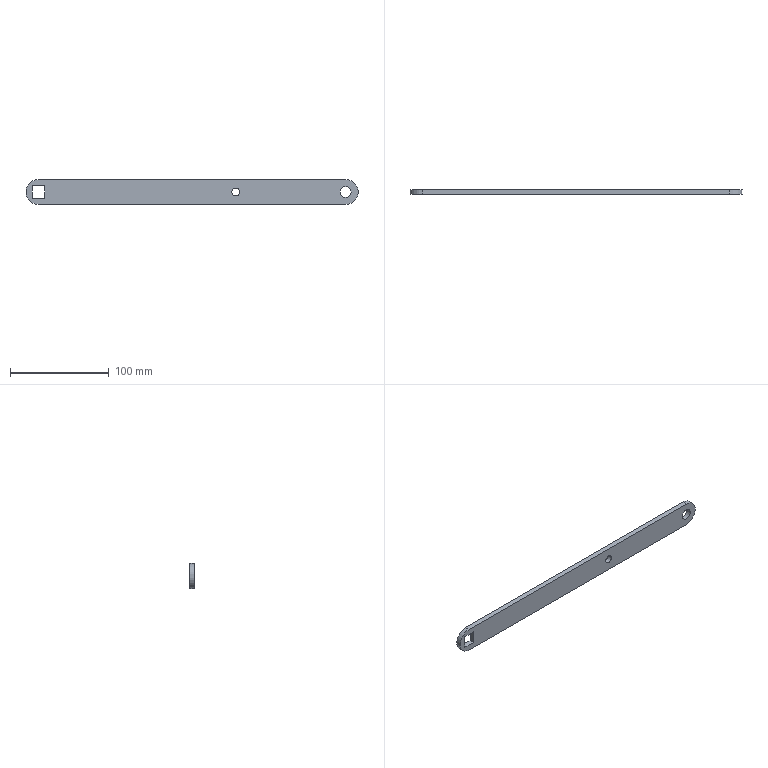Part | NX | features BREP 1 | 1 solid | 18 faces | box 336.55 x 4.763 x 25.4 mm | volume 38541 mm3 | cylinder 10 | plane 8 | commonest cylinder face diameters 0.762 x4 8.128 x2 11.151 x2 25.4 x2
STEP:
#1=CARTESIAN_POINT('',(-155.575,0.,12.7));
#2=VERTEX_POINT('',#1);
#3=CARTESIAN_POINT('',(155.575,0.,12.7));
#4=VERTEX_POINT('',#3);
#5=CARTESIAN_POINT('',(-155.575,0.,12.7));
#6=DIRECTION('',(1.,0.,0.));
#7=VECTOR('',#6,1000.);
#8=LINE('',#5,#7);
#9=EDGE_CURVE('',#2,#4,#8,.T.);
#10=ORIENTED_EDGE('',*,*,#9,.T.);
#11=CARTESIAN_POINT('',(155.575,0.,-12.7));
#12=VERTEX_POINT('',#11);
#13=CARTESIAN_POINT('',(155.575,0.,0.));
#14=DIRECTION('',(0.,1.,0.));
#15=DIRECTION('',(0.,0.,1.));
#16=AXIS2_PLACEMENT_3D('',#13,#14,#15);
#17=CIRCLE('',#16,12.7);
#18=EDGE_CURVE('',#4,#12,#17,.T.);
#19=ORIENTED_EDGE('',*,*,#18,.T.);
#20=CARTESIAN_POINT('',(-155.575,0.,-12.7));
#21=VERTEX_POINT('',#20);
#22=CARTESIAN_POINT('',(155.575,0.,-12.7));
#23=DIRECTION('',(-1.,0.,0.));
#24=VECTOR('',#23,1000.);
#25=LINE('',#22,#24);
#26=EDGE_CURVE('',#12,#21,#25,.T.);
#27=ORIENTED_EDGE('',*,*,#26,.T.);
#28=CARTESIAN_POINT('',(-155.575,0.,0.));
#29=DIRECTION('',(0.,1.,0.));
#30=DIRECTION('',(0.,0.,-1.));
#31=AXIS2_PLACEMENT_3D('',#28,#29,#30);
#32=CIRCLE('',#31,12.7);
#33=EDGE_CURVE('',#21,#2,#32,.T.);
#34=ORIENTED_EDGE('',*,*,#33,.T.);
#35=EDGE_LOOP('',(#10,#19,#27,#34));
#36=FACE_BOUND('',#35,.T.);
#37=CARTESIAN_POINT('',(150.,0.,0.));
#38=VERTEX_POINT('',#37);
#39=CARTESIAN_POINT('',(161.15,0.,0.));
#40=VERTEX_POINT('',#39);
#41=CARTESIAN_POINT('',(155.575,0.,0.));
#42=DIRECTION('',(0.,-1.,0.));
#43=DIRECTION('',(-1.,0.,0.));
#44=AXIS2_PLACEMENT_3D('',#41,#42,#43);
#45=CIRCLE('',#44,5.575);
#46=EDGE_CURVE('',#38,#40,#45,.T.);
#47=ORIENTED_EDGE('',*,*,#46,.T.);
#48=CARTESIAN_POINT('',(155.575,0.,0.));
#49=DIRECTION('',(0.,-1.,0.));
#50=DIRECTION('',(1.,0.,0.));
#51=AXIS2_PLACEMENT_3D('',#48,#49,#50);
#52=CIRCLE('',#51,5.575);
#53=EDGE_CURVE('',#40,#38,#52,.T.);
#54=ORIENTED_EDGE('',*,*,#53,.T.);
#55=EDGE_LOOP('',(#47,#54));
#56=FACE_BOUND('',#55,.T.);
#57=CARTESIAN_POINT('',(-149.098,0.,6.096));
#58=VERTEX_POINT('',#57);
#59=CARTESIAN_POINT('',(-149.479,0.,6.477));
#60=VERTEX_POINT('',#59);
#61=CARTESIAN_POINT('',(-149.479,0.,6.096));
#62=DIRECTION('',(0.,-1.,0.));
#63=DIRECTION('',(1.,0.,0.));
#64=AXIS2_PLACEMENT_3D('',#61,#62,#63);
#65=CIRCLE('',#64,0.381);
#66=EDGE_CURVE('',#58,#60,#65,.T.);
#67=ORIENTED_EDGE('',*,*,#66,.T.);
#68=CARTESIAN_POINT('',(-161.671,0.,6.477));
#69=VERTEX_POINT('',#68);
#70=CARTESIAN_POINT('',(-149.479,0.,6.477));
#71=DIRECTION('',(-1.,0.,0.));
#72=VECTOR('',#71,1000.);
#73=LINE('',#70,#72);
#74=EDGE_CURVE('',#60,#69,#73,.T.);
#75=ORIENTED_EDGE('',*,*,#74,.T.);
#76=CARTESIAN_POINT('',(-162.052,0.,6.096));
#77=VERTEX_POINT('',#76);
#78=CARTESIAN_POINT('',(-161.671,0.,6.096));
#79=DIRECTION('',(0.,-1.,0.));
#80=DIRECTION('',(0.,0.,1.));
#81=AXIS2_PLACEMENT_3D('',#78,#79,#80);
#82=CIRCLE('',#81,0.381);
#83=EDGE_CURVE('',#69,#77,#82,.T.);
#84=ORIENTED_EDGE('',*,*,#83,.T.);
#85=CARTESIAN_POINT('',(-162.052,0.,-6.096));
#86=VERTEX_POINT('',#85);
#87=CARTESIAN_POINT('',(-162.052,0.,6.096));
#88=DIRECTION('',(0.,0.,-1.));
#89=VECTOR('',#88,1000.);
#90=LINE('',#87,#89);
#91=EDGE_CURVE('',#77,#86,#90,.T.);
#92=ORIENTED_EDGE('',*,*,#91,.T.);
#93=CARTESIAN_POINT('',(-161.671,0.,-6.477));
#94=VERTEX_POINT('',#93);
#95=CARTESIAN_POINT('',(-161.671,0.,-6.096));
#96=DIRECTION('',(0.,-1.,0.));
#97=DIRECTION('',(-1.,0.,0.));
#98=AXIS2_PLACEMENT_3D('',#95,#96,#97);
#99=CIRCLE('',#98,0.381);
#100=EDGE_CURVE('',#86,#94,#99,.T.);
#101=ORIENTED_EDGE('',*,*,#100,.T.);
#102=CARTESIAN_POINT('',(-149.479,0.,-6.477));
#103=VERTEX_POINT('',#102);
#104=CARTESIAN_POINT('',(-161.671,0.,-6.477));
#105=DIRECTION('',(1.,0.,0.));
#106=VECTOR('',#105,1000.);
#107=LINE('',#104,#106);
#108=EDGE_CURVE('',#94,#103,#107,.T.);
#109=ORIENTED_EDGE('',*,*,#108,.T.);
#110=CARTESIAN_POINT('',(-149.098,0.,-6.096));
#111=VERTEX_POINT('',#110);
#112=CARTESIAN_POINT('',(-149.479,0.,-6.096));
#113=DIRECTION('',(0.,-1.,0.));
#114=DIRECTION('',(0.,0.,-1.));
#115=AXIS2_PLACEMENT_3D('',#112,#113,#114);
#116=CIRCLE('',#115,0.381);
#117=EDGE_CURVE('',#103,#111,#116,.T.);
#118=ORIENTED_EDGE('',*,*,#117,.T.);
#119=CARTESIAN_POINT('',(-149.098,0.,-6.096));
#120=DIRECTION('',(0.,0.,1.));
#121=VECTOR('',#120,1000.);
#122=LINE('',#119,#121);
#123=EDGE_CURVE('',#111,#58,#122,.T.);
#124=ORIENTED_EDGE('',*,*,#123,.T.);
#125=EDGE_LOOP('',(#67,#75,#84,#92,#101,#109,#118,#124));
#126=FACE_BOUND('',#125,.T.);
#127=CARTESIAN_POINT('',(40.386,0.,0.));
#128=VERTEX_POINT('',#127);
#129=CARTESIAN_POINT('',(48.514,0.,0.));
#130=VERTEX_POINT('',#129);
#131=CARTESIAN_POINT('',(44.45,0.,0.));
#132=DIRECTION('',(0.,1.,0.));
#133=DIRECTION('',(-1.,0.,0.));
#134=AXIS2_PLACEMENT_3D('',#131,#132,#133);
#135=CIRCLE('',#134,4.064);
#136=EDGE_CURVE('',#128,#130,#135,.T.);
#137=ORIENTED_EDGE('',*,*,#136,.F.);
#138=CARTESIAN_POINT('',(44.45,0.,0.));
#139=DIRECTION('',(0.,1.,0.));
#140=DIRECTION('',(1.,0.,0.));
#141=AXIS2_PLACEMENT_3D('',#138,#139,#140);
#142=CIRCLE('',#141,4.064);
#143=EDGE_CURVE('',#130,#128,#142,.T.);
#144=ORIENTED_EDGE('',*,*,#143,.F.);
#145=EDGE_LOOP('',(#137,#144));
#146=FACE_BOUND('',#145,.T.);
#147=CARTESIAN_POINT('',(0.,0.,0.));
#148=DIRECTION('',(0.,1.,0.));
#149=DIRECTION('',(1.,0.,0.));
#150=AXIS2_PLACEMENT_3D('',#147,#148,#149);
#151=PLANE('',#150);
#152=ADVANCED_FACE('',(#36,#56,#126,#146),#151,.T.);
#153=CARTESIAN_POINT('',(-155.575,-4.763,-12.7));
#154=VERTEX_POINT('',#153);
#155=CARTESIAN_POINT('',(-155.575,0.,-12.7));
#156=DIRECTION('',(0.,-1.,0.));
#157=VECTOR('',#156,1000.);
#158=LINE('',#155,#157);
#159=EDGE_CURVE('',#21,#154,#158,.T.);
#160=ORIENTED_EDGE('',*,*,#159,.T.);
#161=CARTESIAN_POINT('',(-155.575,-4.763,12.7));
#162=VERTEX_POINT('',#161);
#163=CARTESIAN_POINT('',(-155.575,-4.763,0.));
#164=DIRECTION('',(0.,1.,0.));
#165=DIRECTION('',(0.,0.,-1.));
#166=AXIS2_PLACEMENT_3D('',#163,#164,#165);
#167=CIRCLE('',#166,12.7);
#168=EDGE_CURVE('',#154,#162,#167,.T.);
#169=ORIENTED_EDGE('',*,*,#168,.T.);
#170=CARTESIAN_POINT('',(-155.575,0.,12.7));
#171=DIRECTION('',(0.,-1.,0.));
#172=VECTOR('',#171,1000.);
#173=LINE('',#170,#172);
#174=EDGE_CURVE('',#2,#162,#173,.T.);
#175=ORIENTED_EDGE('',*,*,#174,.F.);
#176=ORIENTED_EDGE('',*,*,#33,.F.);
#177=EDGE_LOOP('',(#160,#169,#175,#176));
#178=FACE_BOUND('',#177,.T.);
#179=CARTESIAN_POINT('',(-155.575,-2.381,0.));
#180=DIRECTION('',(0.,1.,0.));
#181=DIRECTION('',(0.,0.,-1.));
#182=AXIS2_PLACEMENT_3D('',#179,#180,#181);
#183=CYLINDRICAL_SURFACE('',#182,12.7);
#184=ADVANCED_FACE('',(#178),#183,.T.);
#185=ORIENTED_EDGE('',*,*,#174,.T.);
#186=CARTESIAN_POINT('',(155.575,-4.763,12.7));
#187=VERTEX_POINT('',#186);
#188=CARTESIAN_POINT('',(-155.575,-4.763,12.7));
#189=DIRECTION('',(1.,0.,0.));
#190=VECTOR('',#189,1000.);
#191=LINE('',#188,#190);
#192=EDGE_CURVE('',#162,#187,#191,.T.);
#193=ORIENTED_EDGE('',*,*,#192,.T.);
#194=CARTESIAN_POINT('',(155.575,0.,12.7));
#195=DIRECTION('',(0.,-1.,0.));
#196=VECTOR('',#195,1000.);
#197=LINE('',#194,#196);
#198=EDGE_CURVE('',#4,#187,#197,.T.);
#199=ORIENTED_EDGE('',*,*,#198,.F.);
#200=ORIENTED_EDGE('',*,*,#9,.F.);
#201=EDGE_LOOP('',(#185,#193,#199,#200));
#202=FACE_BOUND('',#201,.T.);
#203=CARTESIAN_POINT('',(0.,-2.381,12.7));
#204=DIRECTION('',(0.,0.,1.));
#205=DIRECTION('',(1.,0.,0.));
#206=AXIS2_PLACEMENT_3D('',#203,#204,#205);
#207=PLANE('',#206);
#208=ADVANCED_FACE('',(#202),#207,.T.);
#209=ORIENTED_EDGE('',*,*,#198,.T.);
#210=CARTESIAN_POINT('',(155.575,-4.763,-12.7));
#211=VERTEX_POINT('',#210);
#212=CARTESIAN_POINT('',(155.575,-4.763,0.));
#213=DIRECTION('',(0.,1.,0.));
#214=DIRECTION('',(0.,0.,1.));
#215=AXIS2_PLACEMENT_3D('',#212,#213,#214);
#216=CIRCLE('',#215,12.7);
#217=EDGE_CURVE('',#187,#211,#216,.T.);
#218=ORIENTED_EDGE('',*,*,#217,.T.);
#219=CARTESIAN_POINT('',(155.575,0.,-12.7));
#220=DIRECTION('',(0.,-1.,0.));
#221=VECTOR('',#220,1000.);
#222=LINE('',#219,#221);
#223=EDGE_CURVE('',#12,#211,#222,.T.);
#224=ORIENTED_EDGE('',*,*,#223,.F.);
#225=ORIENTED_EDGE('',*,*,#18,.F.);
#226=EDGE_LOOP('',(#209,#218,#224,#225));
#227=FACE_BOUND('',#226,.T.);
#228=CARTESIAN_POINT('',(155.575,-2.381,0.));
#229=DIRECTION('',(0.,1.,0.));
#230=DIRECTION('',(0.,0.,1.));
#231=AXIS2_PLACEMENT_3D('',#228,#229,#230);
#232=CYLINDRICAL_SURFACE('',#231,12.7);
#233=ADVANCED_FACE('',(#227),#232,.T.);
#234=ORIENTED_EDGE('',*,*,#223,.T.);
#235=CARTESIAN_POINT('',(155.575,-4.763,-12.7));
#236=DIRECTION('',(-1.,0.,0.));
#237=VECTOR('',#236,1000.);
#238=LINE('',#235,#237);
#239=EDGE_CURVE('',#211,#154,#238,.T.);
#240=ORIENTED_EDGE('',*,*,#239,.T.);
#241=ORIENTED_EDGE('',*,*,#159,.F.);
#242=ORIENTED_EDGE('',*,*,#26,.F.);
#243=EDGE_LOOP('',(#234,#240,#241,#242));
#244=FACE_BOUND('',#243,.T.);
#245=CARTESIAN_POINT('',(0.,-2.381,-12.7));
#246=DIRECTION('',(0.,0.,-1.));
#247=DIRECTION('',(0.,-1.,0.));
#248=AXIS2_PLACEMENT_3D('',#245,#246,#247);
#249=PLANE('',#248);
#250=ADVANCED_FACE('',(#244),#249,.T.);
#251=ORIENTED_EDGE('',*,*,#239,.F.);
#252=ORIENTED_EDGE('',*,*,#217,.F.);
#253=ORIENTED_EDGE('',*,*,#192,.F.);
#254=ORIENTED_EDGE('',*,*,#168,.F.);
#255=EDGE_LOOP('',(#251,#252,#253,#254));
#256=FACE_BOUND('',#255,.T.);
#257=CARTESIAN_POINT('',(150.,-4.763,0.));
#258=VERTEX_POINT('',#257);
#259=CARTESIAN_POINT('',(161.15,-4.763,0.));
#260=VERTEX_POINT('',#259);
#261=CARTESIAN_POINT('',(155.575,-4.763,0.));
#262=DIRECTION('',(0.,-1.,0.));
#263=DIRECTION('',(-1.,0.,0.));
#264=AXIS2_PLACEMENT_3D('',#261,#262,#263);
#265=CIRCLE('',#264,5.575);
#266=EDGE_CURVE('',#258,#260,#265,.T.);
#267=ORIENTED_EDGE('',*,*,#266,.F.);
#268=CARTESIAN_POINT('',(155.575,-4.763,0.));
#269=DIRECTION('',(0.,-1.,0.));
#270=DIRECTION('',(1.,0.,0.));
#271=AXIS2_PLACEMENT_3D('',#268,#269,#270);
#272=CIRCLE('',#271,5.575);
#273=EDGE_CURVE('',#260,#258,#272,.T.);
#274=ORIENTED_EDGE('',*,*,#273,.F.);
#275=EDGE_LOOP('',(#267,#274));
#276=FACE_BOUND('',#275,.T.);
#277=CARTESIAN_POINT('',(-161.671,-4.763,-6.477));
#278=VERTEX_POINT('',#277);
#279=CARTESIAN_POINT('',(-162.052,-4.763,-6.096));
#280=VERTEX_POINT('',#279);
#281=CARTESIAN_POINT('',(-161.671,-4.763,-6.096));
#282=DIRECTION('',(0.,1.,0.));
#283=DIRECTION('',(0.,0.,-1.));
#284=AXIS2_PLACEMENT_3D('',#281,#282,#283);
#285=CIRCLE('',#284,0.381);
#286=EDGE_CURVE('',#278,#280,#285,.T.);
#287=ORIENTED_EDGE('',*,*,#286,.T.);
#288=CARTESIAN_POINT('',(-162.052,-4.763,6.096));
#289=VERTEX_POINT('',#288);
#290=CARTESIAN_POINT('',(-162.052,-4.763,6.096));
#291=DIRECTION('',(0.,0.,-1.));
#292=VECTOR('',#291,1000.);
#293=LINE('',#290,#292);
#294=EDGE_CURVE('',#289,#280,#293,.T.);
#295=ORIENTED_EDGE('',*,*,#294,.F.);
#296=CARTESIAN_POINT('',(-161.671,-4.763,6.477));
#297=VERTEX_POINT('',#296);
#298=CARTESIAN_POINT('',(-161.671,-4.763,6.096));
#299=DIRECTION('',(0.,1.,0.));
#300=DIRECTION('',(-1.,0.,0.));
#301=AXIS2_PLACEMENT_3D('',#298,#299,#300);
#302=CIRCLE('',#301,0.381);
#303=EDGE_CURVE('',#289,#297,#302,.T.);
#304=ORIENTED_EDGE('',*,*,#303,.T.);
#305=CARTESIAN_POINT('',(-149.479,-4.763,6.477));
#306=VERTEX_POINT('',#305);
#307=CARTESIAN_POINT('',(-149.479,-4.763,6.477));
#308=DIRECTION('',(-1.,0.,0.));
#309=VECTOR('',#308,1000.);
#310=LINE('',#307,#309);
#311=EDGE_CURVE('',#306,#297,#310,.T.);
#312=ORIENTED_EDGE('',*,*,#311,.F.);
#313=CARTESIAN_POINT('',(-149.098,-4.763,6.096));
#314=VERTEX_POINT('',#313);
#315=CARTESIAN_POINT('',(-149.479,-4.763,6.096));
#316=DIRECTION('',(0.,1.,0.));
#317=DIRECTION('',(0.,0.,1.));
#318=AXIS2_PLACEMENT_3D('',#315,#316,#317);
#319=CIRCLE('',#318,0.381);
#320=EDGE_CURVE('',#306,#314,#319,.T.);
#321=ORIENTED_EDGE('',*,*,#320,.T.);
#322=CARTESIAN_POINT('',(-149.098,-4.763,-6.096));
#323=VERTEX_POINT('',#322);
#324=CARTESIAN_POINT('',(-149.098,-4.763,-6.096));
#325=DIRECTION('',(0.,0.,1.));
#326=VECTOR('',#325,1000.);
#327=LINE('',#324,#326);
#328=EDGE_CURVE('',#323,#314,#327,.T.);
#329=ORIENTED_EDGE('',*,*,#328,.F.);
#330=CARTESIAN_POINT('',(-149.479,-4.763,-6.477));
#331=VERTEX_POINT('',#330);
#332=CARTESIAN_POINT('',(-149.479,-4.763,-6.096));
#333=DIRECTION('',(0.,1.,0.));
#334=DIRECTION('',(1.,0.,0.));
#335=AXIS2_PLACEMENT_3D('',#332,#333,#334);
#336=CIRCLE('',#335,0.381);
#337=EDGE_CURVE('',#323,#331,#336,.T.);
#338=ORIENTED_EDGE('',*,*,#337,.T.);
#339=CARTESIAN_POINT('',(-161.671,-4.763,-6.477));
#340=DIRECTION('',(1.,0.,0.));
#341=VECTOR('',#340,1000.);
#342=LINE('',#339,#341);
#343=EDGE_CURVE('',#278,#331,#342,.T.);
#344=ORIENTED_EDGE('',*,*,#343,.F.);
#345=EDGE_LOOP('',(#287,#295,#304,#312,#321,#329,#338,#344));
#346=FACE_BOUND('',#345,.T.);
#347=CARTESIAN_POINT('',(40.386,-4.763,0.));
#348=VERTEX_POINT('',#347);
#349=CARTESIAN_POINT('',(48.514,-4.763,0.));
#350=VERTEX_POINT('',#349);
#351=CARTESIAN_POINT('',(44.45,-4.763,0.));
#352=DIRECTION('',(0.,1.,0.));
#353=DIRECTION('',(-1.,0.,0.));
#354=AXIS2_PLACEMENT_3D('',#351,#352,#353);
#355=CIRCLE('',#354,4.064);
#356=EDGE_CURVE('',#348,#350,#355,.T.);
#357=ORIENTED_EDGE('',*,*,#356,.T.);
#358=CARTESIAN_POINT('',(44.45,-4.763,0.));
#359=DIRECTION('',(0.,1.,0.));
#360=DIRECTION('',(1.,0.,0.));
#361=AXIS2_PLACEMENT_3D('',#358,#359,#360);
#362=CIRCLE('',#361,4.064);
#363=EDGE_CURVE('',#350,#348,#362,.T.);
#364=ORIENTED_EDGE('',*,*,#363,.T.);
#365=EDGE_LOOP('',(#357,#364));
#366=FACE_BOUND('',#365,.T.);
#367=CARTESIAN_POINT('',(0.,-4.763,0.));
#368=DIRECTION('',(0.,1.,0.));
#369=DIRECTION('',(1.,0.,0.));
#370=AXIS2_PLACEMENT_3D('',#367,#368,#369);
#371=PLANE('',#370);
#372=ADVANCED_FACE('',(#256,#276,#346,#366),#371,.F.);
#373=CARTESIAN_POINT('',(161.15,0.,0.));
#374=DIRECTION('',(0.,-1.,0.));
#375=VECTOR('',#374,1000.);
#376=LINE('',#373,#375);
#377=EDGE_CURVE('',#260,#40,#376,.F.);
#378=ORIENTED_EDGE('',*,*,#377,.F.);
#379=ORIENTED_EDGE('',*,*,#273,.T.);
#380=CARTESIAN_POINT('',(150.,0.,0.));
#381=DIRECTION('',(0.,-1.,0.));
#382=VECTOR('',#381,1000.);
#383=LINE('',#380,#382);
#384=EDGE_CURVE('',#258,#38,#383,.F.);
#385=ORIENTED_EDGE('',*,*,#384,.T.);
#386=ORIENTED_EDGE('',*,*,#53,.F.);
#387=EDGE_LOOP('',(#378,#379,#385,#386));
#388=FACE_BOUND('',#387,.T.);
#389=CARTESIAN_POINT('',(155.575,0.,0.));
#390=DIRECTION('',(0.,-1.,0.));
#391=DIRECTION('',(1.,0.,0.));
#392=AXIS2_PLACEMENT_3D('',#389,#390,#391);
#393=CYLINDRICAL_SURFACE('',#392,5.575);
#394=ADVANCED_FACE('',(#388),#393,.F.);
#395=ORIENTED_EDGE('',*,*,#384,.F.);
#396=ORIENTED_EDGE('',*,*,#266,.T.);
#397=ORIENTED_EDGE('',*,*,#377,.T.);
#398=ORIENTED_EDGE('',*,*,#46,.F.);
#399=EDGE_LOOP('',(#395,#396,#397,#398));
#400=FACE_BOUND('',#399,.T.);
#401=CARTESIAN_POINT('',(155.575,0.,0.));
#402=DIRECTION('',(0.,-1.,0.));
#403=DIRECTION('',(1.,0.,0.));
#404=AXIS2_PLACEMENT_3D('',#401,#402,#403);
#405=CYLINDRICAL_SURFACE('',#404,5.575);
#406=ADVANCED_FACE('',(#400),#405,.F.);
#407=ORIENTED_EDGE('',*,*,#343,.T.);
#408=CARTESIAN_POINT('',(-149.479,0.,-6.477));
#409=DIRECTION('',(0.,-1.,0.));
#410=VECTOR('',#409,1000.);
#411=LINE('',#408,#410);
#412=EDGE_CURVE('',#103,#331,#411,.T.);
#413=ORIENTED_EDGE('',*,*,#412,.F.);
#414=ORIENTED_EDGE('',*,*,#108,.F.);
#415=CARTESIAN_POINT('',(-161.671,0.,-6.477));
#416=DIRECTION('',(0.,-1.,0.));
#417=VECTOR('',#416,1000.);
#418=LINE('',#415,#417);
#419=EDGE_CURVE('',#94,#278,#418,.T.);
#420=ORIENTED_EDGE('',*,*,#419,.T.);
#421=EDGE_LOOP('',(#407,#413,#414,#420));
#422=FACE_BOUND('',#421,.T.);
#423=CARTESIAN_POINT('',(-155.575,-2.381,-6.477));
#424=DIRECTION('',(0.,0.,1.));
#425=DIRECTION('',(1.,0.,0.));
#426=AXIS2_PLACEMENT_3D('',#423,#424,#425);
#427=PLANE('',#426);
#428=ADVANCED_FACE('',(#422),#427,.T.);
#429=ORIENTED_EDGE('',*,*,#286,.F.);
#430=ORIENTED_EDGE('',*,*,#419,.F.);
#431=ORIENTED_EDGE('',*,*,#100,.F.);
#432=CARTESIAN_POINT('',(-162.052,0.,-6.096));
#433=DIRECTION('',(0.,-1.,0.));
#434=VECTOR('',#433,1000.);
#435=LINE('',#432,#434);
#436=EDGE_CURVE('',#86,#280,#435,.T.);
#437=ORIENTED_EDGE('',*,*,#436,.T.);
#438=EDGE_LOOP('',(#429,#430,#431,#437));
#439=FACE_BOUND('',#438,.T.);
#440=CARTESIAN_POINT('',(-161.671,0.5809,-6.096));
#441=DIRECTION('',(0.,-1.,0.));
#442=DIRECTION('',(-1.,0.,0.));
#443=AXIS2_PLACEMENT_3D('',#440,#441,#442);
#444=CYLINDRICAL_SURFACE('',#443,0.381);
#445=ADVANCED_FACE('',(#439),#444,.F.);
#446=ORIENTED_EDGE('',*,*,#91,.F.);
#447=CARTESIAN_POINT('',(-162.052,0.,6.096));
#448=DIRECTION('',(0.,-1.,0.));
#449=VECTOR('',#448,1000.);
#450=LINE('',#447,#449);
#451=EDGE_CURVE('',#77,#289,#450,.T.);
#452=ORIENTED_EDGE('',*,*,#451,.T.);
#453=ORIENTED_EDGE('',*,*,#294,.T.);
#454=ORIENTED_EDGE('',*,*,#436,.F.);
#455=EDGE_LOOP('',(#446,#452,#453,#454));
#456=FACE_BOUND('',#455,.T.);
#457=CARTESIAN_POINT('',(-162.052,-2.381,0.));
#458=DIRECTION('',(1.,0.,0.));
#459=DIRECTION('',(0.,1.,0.));
#460=AXIS2_PLACEMENT_3D('',#457,#458,#459);
#461=PLANE('',#460);
#462=ADVANCED_FACE('',(#456),#461,.T.);
#463=ORIENTED_EDGE('',*,*,#303,.F.);
#464=ORIENTED_EDGE('',*,*,#451,.F.);
#465=ORIENTED_EDGE('',*,*,#83,.F.);
#466=CARTESIAN_POINT('',(-161.671,0.,6.477));
#467=DIRECTION('',(0.,-1.,0.));
#468=VECTOR('',#467,1000.);
#469=LINE('',#466,#468);
#470=EDGE_CURVE('',#69,#297,#469,.T.);
#471=ORIENTED_EDGE('',*,*,#470,.T.);
#472=EDGE_LOOP('',(#463,#464,#465,#471));
#473=FACE_BOUND('',#472,.T.);
#474=CARTESIAN_POINT('',(-161.671,0.5809,6.096));
#475=DIRECTION('',(0.,-1.,0.));
#476=DIRECTION('',(0.,0.,1.));
#477=AXIS2_PLACEMENT_3D('',#474,#475,#476);
#478=CYLINDRICAL_SURFACE('',#477,0.381);
#479=ADVANCED_FACE('',(#473),#478,.F.);
#480=ORIENTED_EDGE('',*,*,#311,.T.);
#481=ORIENTED_EDGE('',*,*,#470,.F.);
#482=ORIENTED_EDGE('',*,*,#74,.F.);
#483=CARTESIAN_POINT('',(-149.479,0.,6.477));
#484=DIRECTION('',(0.,-1.,0.));
#485=VECTOR('',#484,1000.);
#486=LINE('',#483,#485);
#487=EDGE_CURVE('',#60,#306,#486,.T.);
#488=ORIENTED_EDGE('',*,*,#487,.T.);
#489=EDGE_LOOP('',(#480,#481,#482,#488));
#490=FACE_BOUND('',#489,.T.);
#491=CARTESIAN_POINT('',(-155.575,-2.381,6.477));
#492=DIRECTION('',(0.,0.,-1.));
#493=DIRECTION('',(0.,-1.,0.));
#494=AXIS2_PLACEMENT_3D('',#491,#492,#493);
#495=PLANE('',#494);
#496=ADVANCED_FACE('',(#490),#495,.T.);
#497=ORIENTED_EDGE('',*,*,#320,.F.);
#498=ORIENTED_EDGE('',*,*,#487,.F.);
#499=ORIENTED_EDGE('',*,*,#66,.F.);
#500=CARTESIAN_POINT('',(-149.098,0.,6.096));
#501=DIRECTION('',(0.,-1.,0.));
#502=VECTOR('',#501,1000.);
#503=LINE('',#500,#502);
#504=EDGE_CURVE('',#58,#314,#503,.T.);
#505=ORIENTED_EDGE('',*,*,#504,.T.);
#506=EDGE_LOOP('',(#497,#498,#499,#505));
#507=FACE_BOUND('',#506,.T.);
#508=CARTESIAN_POINT('',(-149.479,0.5809,6.096));
#509=DIRECTION('',(0.,-1.,0.));
#510=DIRECTION('',(1.,0.,0.));
#511=AXIS2_PLACEMENT_3D('',#508,#509,#510);
#512=CYLINDRICAL_SURFACE('',#511,0.381);
#513=ADVANCED_FACE('',(#507),#512,.F.);
#514=ORIENTED_EDGE('',*,*,#328,.T.);
#515=ORIENTED_EDGE('',*,*,#504,.F.);
#516=ORIENTED_EDGE('',*,*,#123,.F.);
#517=CARTESIAN_POINT('',(-149.098,0.,-6.096));
#518=DIRECTION('',(0.,-1.,0.));
#519=VECTOR('',#518,1000.);
#520=LINE('',#517,#519);
#521=EDGE_CURVE('',#111,#323,#520,.T.);
#522=ORIENTED_EDGE('',*,*,#521,.T.);
#523=EDGE_LOOP('',(#514,#515,#516,#522));
#524=FACE_BOUND('',#523,.T.);
#525=CARTESIAN_POINT('',(-149.098,-2.381,0.));
#526=DIRECTION('',(-1.,0.,0.));
#527=DIRECTION('',(0.,0.,1.));
#528=AXIS2_PLACEMENT_3D('',#525,#526,#527);
#529=PLANE('',#528);
#530=ADVANCED_FACE('',(#524),#529,.T.);
#531=ORIENTED_EDGE('',*,*,#337,.F.);
#532=ORIENTED_EDGE('',*,*,#521,.F.);
#533=ORIENTED_EDGE('',*,*,#117,.F.);
#534=ORIENTED_EDGE('',*,*,#412,.T.);
#535=EDGE_LOOP('',(#531,#532,#533,#534));
#536=FACE_BOUND('',#535,.T.);
#537=CARTESIAN_POINT('',(-149.479,0.5809,-6.096));
#538=DIRECTION('',(0.,-1.,0.));
#539=DIRECTION('',(0.,0.,-1.));
#540=AXIS2_PLACEMENT_3D('',#537,#538,#539);
#541=CYLINDRICAL_SURFACE('',#540,0.381);
#542=ADVANCED_FACE('',(#536),#541,.F.);
#543=CARTESIAN_POINT('',(40.386,0.,0.));
#544=DIRECTION('',(0.,-1.,0.));
#545=VECTOR('',#544,1000.);
#546=LINE('',#543,#545);
#547=EDGE_CURVE('',#128,#348,#546,.T.);
#548=ORIENTED_EDGE('',*,*,#547,.T.);
#549=ORIENTED_EDGE('',*,*,#363,.F.);
#550=CARTESIAN_POINT('',(48.514,0.,0.));
#551=DIRECTION('',(0.,-1.,0.));
#552=VECTOR('',#551,1000.);
#553=LINE('',#550,#552);
#554=EDGE_CURVE('',#130,#350,#553,.T.);
#555=ORIENTED_EDGE('',*,*,#554,.F.);
#556=ORIENTED_EDGE('',*,*,#143,.T.);
#557=EDGE_LOOP('',(#548,#549,#555,#556));
#558=FACE_BOUND('',#557,.T.);
#559=CARTESIAN_POINT('',(44.45,-2.381,0.));
#560=DIRECTION('',(0.,1.,0.));
#561=DIRECTION('',(1.,0.,0.));
#562=AXIS2_PLACEMENT_3D('',#559,#560,#561);
#563=CYLINDRICAL_SURFACE('',#562,4.064);
#564=ADVANCED_FACE('',(#558),#563,.F.);
#565=ORIENTED_EDGE('',*,*,#554,.T.);
#566=ORIENTED_EDGE('',*,*,#356,.F.);
#567=ORIENTED_EDGE('',*,*,#547,.F.);
#568=ORIENTED_EDGE('',*,*,#136,.T.);
#569=EDGE_LOOP('',(#565,#566,#567,#568));
#570=FACE_BOUND('',#569,.T.);
#571=CARTESIAN_POINT('',(44.45,-2.381,0.));
#572=DIRECTION('',(0.,1.,0.));
#573=DIRECTION('',(-1.,0.,0.));
#574=AXIS2_PLACEMENT_3D('',#571,#572,#573);
#575=CYLINDRICAL_SURFACE('',#574,4.064);
#576=ADVANCED_FACE('',(#570),#575,.F.);
#577=CLOSED_SHELL('',(#152,#184,#208,#233,#250,#372,#394,#406,#428,#445,#462,#479,#496,#513,#530,#542,#564,#576));
#578=MANIFOLD_SOLID_BREP('',#577);
#579=(LENGTH_UNIT()NAMED_UNIT(*)SI_UNIT(.MILLI.,.METRE.));
#580=UNCERTAINTY_MEASURE_WITH_UNIT(LENGTH_MEASURE(0.00001),#579,'','');
#581=(NAMED_UNIT(*)PLANE_ANGLE_UNIT()SI_UNIT($,.RADIAN.));
#582=(NAMED_UNIT(*)SI_UNIT($,.STERADIAN.)SOLID_ANGLE_UNIT());
#583=(GEOMETRIC_REPRESENTATION_CONTEXT(3)GLOBAL_UNCERTAINTY_ASSIGNED_CONTEXT((#580))GLOBAL_UNIT_ASSIGNED_CONTEXT((#579,#581,#582))REPRESENTATION_CONTEXT('',''));
#584=ADVANCED_BREP_SHAPE_REPRESENTATION('',(#578),#583);